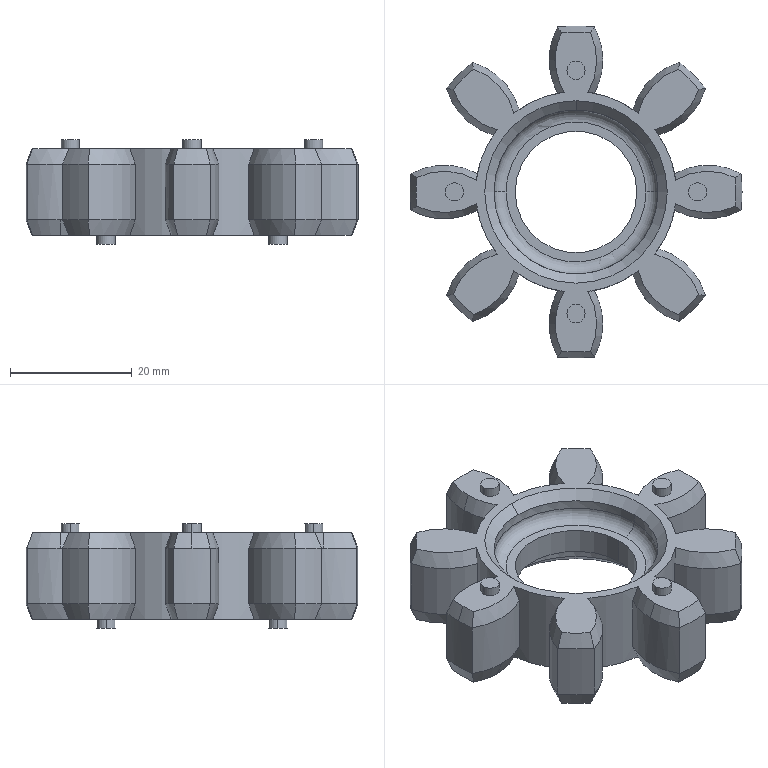Part | NX | features BREP 1 | 1 solid | 132 faces | box 54.6 x 54.6 x 17.2 mm | volume 14306 mm3 | cone 59 | cylinder 57 | plane 12 | torus 4 | commonest cylinder face diameters 22.654 x18 3 x16 54.6 x9 33 x8 27 x4 20 x2